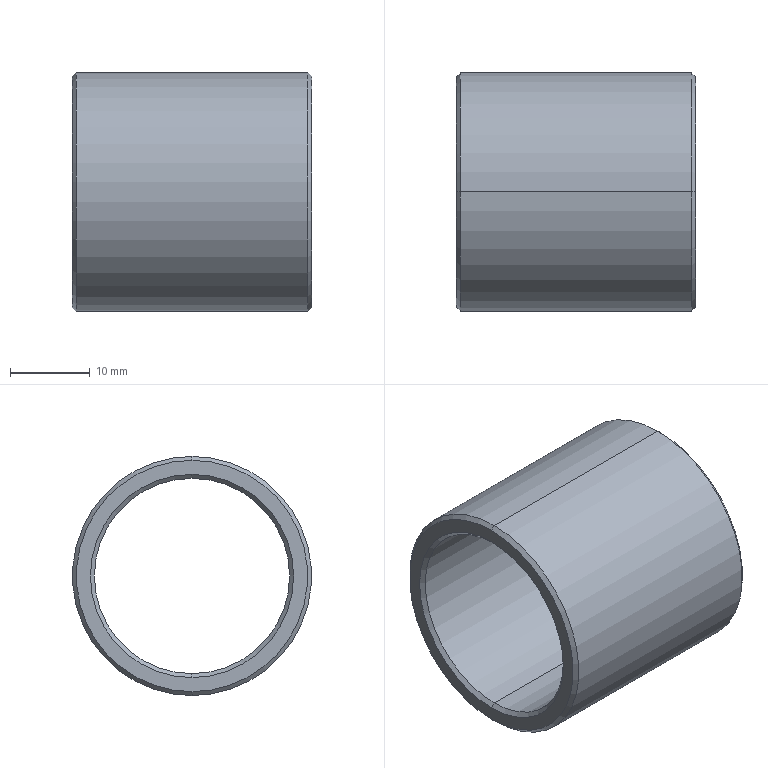Part | SolidWorks | features Revolution 1 | 1 solid | 14 faces | box 30 x 30 x 30 mm | volume 7020 mm3 | cone 8 | cylinder 4 | plane 2 | commonest cylinder face diameters 24.5 x2 30 x2
STEP:
#1=CARTESIAN_POINT('',(-14.5,0.,-12.25));
#2=VERTEX_POINT('',#1);
#3=CARTESIAN_POINT('',(-14.5,0.,12.25));
#4=VERTEX_POINT('',#3);
#5=CARTESIAN_POINT('',(-14.5,0.,0.));
#6=DIRECTION('',(-1.,0.,0.));
#7=DIRECTION('',(0.,0.,1.));
#8=AXIS2_PLACEMENT_3D('',#5,#6,#7);
#9=CIRCLE('',#8,12.25);
#10=EDGE_CURVE('',#2,#4,#9,.T.);
#11=ORIENTED_EDGE('',*,*,#10,.F.);
#12=CARTESIAN_POINT('',(-15.,0.,-12.75));
#13=VERTEX_POINT('',#12);
#14=CARTESIAN_POINT('',(-15.,0.,-12.75));
#15=DIRECTION('',(-0.7071,0.,-0.7071));
#16=VECTOR('',#15,1000.);
#17=LINE('',#14,#16);
#18=EDGE_CURVE('',#2,#13,#17,.T.);
#19=ORIENTED_EDGE('',*,*,#18,.T.);
#20=CARTESIAN_POINT('',(-15.,0.,12.75));
#21=VERTEX_POINT('',#20);
#22=CARTESIAN_POINT('',(-15.,0.,0.));
#23=DIRECTION('',(-1.,0.,0.));
#24=DIRECTION('',(0.,0.,1.));
#25=AXIS2_PLACEMENT_3D('',#22,#23,#24);
#26=CIRCLE('',#25,12.75);
#27=EDGE_CURVE('',#13,#21,#26,.T.);
#28=ORIENTED_EDGE('',*,*,#27,.T.);
#29=CARTESIAN_POINT('',(-15.,0.,12.75));
#30=DIRECTION('',(-0.7071,0.,0.7071));
#31=VECTOR('',#30,1000.);
#32=LINE('',#29,#31);
#33=EDGE_CURVE('',#4,#21,#32,.T.);
#34=ORIENTED_EDGE('',*,*,#33,.F.);
#35=EDGE_LOOP('',(#11,#19,#28,#34));
#36=FACE_OUTER_BOUND('',#35,.T.);
#37=CARTESIAN_POINT('',(-15.,0.,0.));
#38=DIRECTION('',(-1.,0.,0.));
#39=DIRECTION('',(0.,0.,1.));
#40=AXIS2_PLACEMENT_3D('',#37,#38,#39);
#41=CONICAL_SURFACE('',#40,12.75,0.7854);
#42=ADVANCED_FACE('',(#36),#41,.F.);
#43=CARTESIAN_POINT('',(14.5,0.,-12.25));
#44=VERTEX_POINT('',#43);
#45=CARTESIAN_POINT('',(14.5,0.,12.25));
#46=VERTEX_POINT('',#45);
#47=CARTESIAN_POINT('',(14.5,0.,0.));
#48=DIRECTION('',(-1.,0.,0.));
#49=DIRECTION('',(0.,0.,1.));
#50=AXIS2_PLACEMENT_3D('',#47,#48,#49);
#51=CIRCLE('',#50,12.25);
#52=EDGE_CURVE('',#44,#46,#51,.T.);
#53=ORIENTED_EDGE('',*,*,#52,.F.);
#54=CARTESIAN_POINT('',(-1000.,0.,-12.25));
#55=DIRECTION('',(-1.,0.,0.));
#56=VECTOR('',#55,1000.);
#57=LINE('',#54,#56);
#58=EDGE_CURVE('',#44,#2,#57,.T.);
#59=ORIENTED_EDGE('',*,*,#58,.T.);
#60=ORIENTED_EDGE('',*,*,#10,.T.);
#61=CARTESIAN_POINT('',(-1000.,0.,12.25));
#62=DIRECTION('',(-1.,0.,0.));
#63=VECTOR('',#62,1000.);
#64=LINE('',#61,#63);
#65=EDGE_CURVE('',#46,#4,#64,.T.);
#66=ORIENTED_EDGE('',*,*,#65,.F.);
#67=EDGE_LOOP('',(#53,#59,#60,#66));
#68=FACE_OUTER_BOUND('',#67,.T.);
#69=CARTESIAN_POINT('',(-1000.,0.,0.));
#70=DIRECTION('',(-1.,0.,0.));
#71=DIRECTION('',(0.,0.,1.));
#72=AXIS2_PLACEMENT_3D('',#69,#70,#71);
#73=CYLINDRICAL_SURFACE('',#72,12.25);
#74=ADVANCED_FACE('',(#68),#73,.F.);
#75=ORIENTED_EDGE('',*,*,#52,.T.);
#76=CARTESIAN_POINT('',(15.,0.,12.75));
#77=VERTEX_POINT('',#76);
#78=CARTESIAN_POINT('',(14.5,0.,12.25));
#79=DIRECTION('',(0.7071,0.,0.7071));
#80=VECTOR('',#79,1000.);
#81=LINE('',#78,#80);
#82=EDGE_CURVE('',#46,#77,#81,.T.);
#83=ORIENTED_EDGE('',*,*,#82,.T.);
#84=CARTESIAN_POINT('',(15.,0.,-12.75));
#85=VERTEX_POINT('',#84);
#86=CARTESIAN_POINT('',(15.,0.,0.));
#87=DIRECTION('',(-1.,0.,0.));
#88=DIRECTION('',(0.,0.,1.));
#89=AXIS2_PLACEMENT_3D('',#86,#87,#88);
#90=CIRCLE('',#89,12.75);
#91=EDGE_CURVE('',#85,#77,#90,.T.);
#92=ORIENTED_EDGE('',*,*,#91,.F.);
#93=CARTESIAN_POINT('',(14.5,0.,-12.25));
#94=DIRECTION('',(0.7071,0.,-0.7071));
#95=VECTOR('',#94,1000.);
#96=LINE('',#93,#95);
#97=EDGE_CURVE('',#44,#85,#96,.T.);
#98=ORIENTED_EDGE('',*,*,#97,.F.);
#99=EDGE_LOOP('',(#75,#83,#92,#98));
#100=FACE_OUTER_BOUND('',#99,.T.);
#101=CARTESIAN_POINT('',(14.5,0.,0.));
#102=DIRECTION('',(1.,0.,0.));
#103=DIRECTION('',(0.,0.,-1.));
#104=AXIS2_PLACEMENT_3D('',#101,#102,#103);
#105=CONICAL_SURFACE('',#104,12.25,0.7854);
#106=ADVANCED_FACE('',(#100),#105,.F.);
#107=CARTESIAN_POINT('',(15.,0.,14.5));
#108=VERTEX_POINT('',#107);
#109=CARTESIAN_POINT('',(15.,0.,-14.5));
#110=VERTEX_POINT('',#109);
#111=CARTESIAN_POINT('',(15.,0.,0.));
#112=DIRECTION('',(-1.,0.,0.));
#113=DIRECTION('',(0.,0.,1.));
#114=AXIS2_PLACEMENT_3D('',#111,#112,#113);
#115=CIRCLE('',#114,14.5);
#116=EDGE_CURVE('',#108,#110,#115,.T.);
#117=ORIENTED_EDGE('',*,*,#116,.T.);
#118=CARTESIAN_POINT('',(14.5,0.,-15.));
#119=VERTEX_POINT('',#118);
#120=CARTESIAN_POINT('',(15.,0.,-14.5));
#121=DIRECTION('',(-0.7071,0.,-0.7071));
#122=VECTOR('',#121,1000.);
#123=LINE('',#120,#122);
#124=EDGE_CURVE('',#110,#119,#123,.T.);
#125=ORIENTED_EDGE('',*,*,#124,.T.);
#126=CARTESIAN_POINT('',(14.5,0.,15.));
#127=VERTEX_POINT('',#126);
#128=CARTESIAN_POINT('',(14.5,0.,0.));
#129=DIRECTION('',(-1.,0.,0.));
#130=DIRECTION('',(0.,0.,1.));
#131=AXIS2_PLACEMENT_3D('',#128,#129,#130);
#132=CIRCLE('',#131,15.);
#133=EDGE_CURVE('',#127,#119,#132,.T.);
#134=ORIENTED_EDGE('',*,*,#133,.F.);
#135=CARTESIAN_POINT('',(15.,0.,14.5));
#136=DIRECTION('',(-0.7071,0.,0.7071));
#137=VECTOR('',#136,1000.);
#138=LINE('',#135,#137);
#139=EDGE_CURVE('',#108,#127,#138,.T.);
#140=ORIENTED_EDGE('',*,*,#139,.F.);
#141=EDGE_LOOP('',(#117,#125,#134,#140));
#142=FACE_OUTER_BOUND('',#141,.T.);
#143=CARTESIAN_POINT('',(15.,0.,0.));
#144=DIRECTION('',(-1.,0.,0.));
#145=DIRECTION('',(0.,0.,1.));
#146=AXIS2_PLACEMENT_3D('',#143,#144,#145);
#147=CONICAL_SURFACE('',#146,14.5,0.7854);
#148=ADVANCED_FACE('',(#142),#147,.T.);
#149=ORIENTED_EDGE('',*,*,#133,.T.);
#150=CARTESIAN_POINT('',(-14.5,0.,-15.));
#151=VERTEX_POINT('',#150);
#152=CARTESIAN_POINT('',(-1000.,0.,-15.));
#153=DIRECTION('',(-1.,0.,0.));
#154=VECTOR('',#153,1000.);
#155=LINE('',#152,#154);
#156=EDGE_CURVE('',#119,#151,#155,.T.);
#157=ORIENTED_EDGE('',*,*,#156,.T.);
#158=CARTESIAN_POINT('',(-14.5,0.,15.));
#159=VERTEX_POINT('',#158);
#160=CARTESIAN_POINT('',(-14.5,0.,0.));
#161=DIRECTION('',(-1.,0.,0.));
#162=DIRECTION('',(0.,0.,1.));
#163=AXIS2_PLACEMENT_3D('',#160,#161,#162);
#164=CIRCLE('',#163,15.);
#165=EDGE_CURVE('',#159,#151,#164,.T.);
#166=ORIENTED_EDGE('',*,*,#165,.F.);
#167=CARTESIAN_POINT('',(-1000.,0.,15.));
#168=DIRECTION('',(-1.,0.,0.));
#169=VECTOR('',#168,1000.);
#170=LINE('',#167,#169);
#171=EDGE_CURVE('',#127,#159,#170,.T.);
#172=ORIENTED_EDGE('',*,*,#171,.F.);
#173=EDGE_LOOP('',(#149,#157,#166,#172));
#174=FACE_OUTER_BOUND('',#173,.T.);
#175=CARTESIAN_POINT('',(-1000.,0.,0.));
#176=DIRECTION('',(-1.,0.,0.));
#177=DIRECTION('',(0.,0.,1.));
#178=AXIS2_PLACEMENT_3D('',#175,#176,#177);
#179=CYLINDRICAL_SURFACE('',#178,15.);
#180=ADVANCED_FACE('',(#174),#179,.T.);
#181=CARTESIAN_POINT('',(-15.,0.,14.5));
#182=VERTEX_POINT('',#181);
#183=CARTESIAN_POINT('',(-15.,0.,-14.5));
#184=VERTEX_POINT('',#183);
#185=CARTESIAN_POINT('',(-15.,0.,0.));
#186=DIRECTION('',(-1.,0.,0.));
#187=DIRECTION('',(0.,0.,1.));
#188=AXIS2_PLACEMENT_3D('',#185,#186,#187);
#189=CIRCLE('',#188,14.5);
#190=EDGE_CURVE('',#182,#184,#189,.T.);
#191=ORIENTED_EDGE('',*,*,#190,.F.);
#192=CARTESIAN_POINT('',(-14.5,0.,15.));
#193=DIRECTION('',(0.7071,0.,0.7071));
#194=VECTOR('',#193,1000.);
#195=LINE('',#192,#194);
#196=EDGE_CURVE('',#182,#159,#195,.T.);
#197=ORIENTED_EDGE('',*,*,#196,.T.);
#198=ORIENTED_EDGE('',*,*,#165,.T.);
#199=CARTESIAN_POINT('',(-14.5,0.,-15.));
#200=DIRECTION('',(0.7071,0.,-0.7071));
#201=VECTOR('',#200,1000.);
#202=LINE('',#199,#201);
#203=EDGE_CURVE('',#184,#151,#202,.T.);
#204=ORIENTED_EDGE('',*,*,#203,.F.);
#205=EDGE_LOOP('',(#191,#197,#198,#204));
#206=FACE_OUTER_BOUND('',#205,.T.);
#207=CARTESIAN_POINT('',(-14.5,0.,0.));
#208=DIRECTION('',(1.,0.,0.));
#209=DIRECTION('',(0.,0.,-1.));
#210=AXIS2_PLACEMENT_3D('',#207,#208,#209);
#211=CONICAL_SURFACE('',#210,15.,0.7854);
#212=ADVANCED_FACE('',(#206),#211,.T.);
#213=CARTESIAN_POINT('',(-15.,0.,0.));
#214=DIRECTION('',(-1.,0.,0.));
#215=DIRECTION('',(0.,0.,1.));
#216=AXIS2_PLACEMENT_3D('',#213,#214,#215);
#217=CIRCLE('',#216,12.75);
#218=EDGE_CURVE('',#21,#13,#217,.T.);
#219=ORIENTED_EDGE('',*,*,#218,.F.);
#220=ORIENTED_EDGE('',*,*,#27,.F.);
#221=EDGE_LOOP('',(#219,#220));
#222=FACE_BOUND('',#221,.T.);
#223=CARTESIAN_POINT('',(-15.,0.,0.));
#224=DIRECTION('',(-1.,0.,0.));
#225=DIRECTION('',(0.,0.,1.));
#226=AXIS2_PLACEMENT_3D('',#223,#224,#225);
#227=CIRCLE('',#226,14.5);
#228=EDGE_CURVE('',#184,#182,#227,.T.);
#229=ORIENTED_EDGE('',*,*,#228,.T.);
#230=ORIENTED_EDGE('',*,*,#190,.T.);
#231=EDGE_LOOP('',(#229,#230));
#232=FACE_OUTER_BOUND('',#231,.T.);
#233=CARTESIAN_POINT('',(-15.,0.,-12.75));
#234=DIRECTION('',(1.,0.,0.));
#235=DIRECTION('',(0.,0.,-1.));
#236=AXIS2_PLACEMENT_3D('',#233,#234,#235);
#237=PLANE('',#236);
#238=ADVANCED_FACE('',(#222,#232),#237,.F.);
#239=ORIENTED_EDGE('',*,*,#196,.F.);
#240=ORIENTED_EDGE('',*,*,#228,.F.);
#241=ORIENTED_EDGE('',*,*,#203,.T.);
#242=CARTESIAN_POINT('',(-14.5,0.,0.));
#243=DIRECTION('',(-1.,0.,0.));
#244=DIRECTION('',(0.,0.,1.));
#245=AXIS2_PLACEMENT_3D('',#242,#243,#244);
#246=CIRCLE('',#245,15.);
#247=EDGE_CURVE('',#151,#159,#246,.T.);
#248=ORIENTED_EDGE('',*,*,#247,.T.);
#249=EDGE_LOOP('',(#239,#240,#241,#248));
#250=FACE_OUTER_BOUND('',#249,.T.);
#251=CARTESIAN_POINT('',(-14.5,0.,0.));
#252=DIRECTION('',(1.,0.,0.));
#253=DIRECTION('',(0.,0.,-1.));
#254=AXIS2_PLACEMENT_3D('',#251,#252,#253);
#255=CONICAL_SURFACE('',#254,15.,0.7854);
#256=ADVANCED_FACE('',(#250),#255,.T.);
#257=ORIENTED_EDGE('',*,*,#156,.F.);
#258=CARTESIAN_POINT('',(14.5,0.,0.));
#259=DIRECTION('',(-1.,0.,0.));
#260=DIRECTION('',(0.,0.,1.));
#261=AXIS2_PLACEMENT_3D('',#258,#259,#260);
#262=CIRCLE('',#261,15.);
#263=EDGE_CURVE('',#119,#127,#262,.T.);
#264=ORIENTED_EDGE('',*,*,#263,.T.);
#265=ORIENTED_EDGE('',*,*,#171,.T.);
#266=ORIENTED_EDGE('',*,*,#247,.F.);
#267=EDGE_LOOP('',(#257,#264,#265,#266));
#268=FACE_OUTER_BOUND('',#267,.T.);
#269=CARTESIAN_POINT('',(-1000.,0.,0.));
#270=DIRECTION('',(-1.,0.,0.));
#271=DIRECTION('',(0.,0.,1.));
#272=AXIS2_PLACEMENT_3D('',#269,#270,#271);
#273=CYLINDRICAL_SURFACE('',#272,15.);
#274=ADVANCED_FACE('',(#268),#273,.T.);
#275=ORIENTED_EDGE('',*,*,#124,.F.);
#276=CARTESIAN_POINT('',(15.,0.,0.));
#277=DIRECTION('',(-1.,0.,0.));
#278=DIRECTION('',(0.,0.,1.));
#279=AXIS2_PLACEMENT_3D('',#276,#277,#278);
#280=CIRCLE('',#279,14.5);
#281=EDGE_CURVE('',#110,#108,#280,.T.);
#282=ORIENTED_EDGE('',*,*,#281,.T.);
#283=ORIENTED_EDGE('',*,*,#139,.T.);
#284=ORIENTED_EDGE('',*,*,#263,.F.);
#285=EDGE_LOOP('',(#275,#282,#283,#284));
#286=FACE_OUTER_BOUND('',#285,.T.);
#287=CARTESIAN_POINT('',(15.,0.,0.));
#288=DIRECTION('',(-1.,0.,0.));
#289=DIRECTION('',(0.,0.,1.));
#290=AXIS2_PLACEMENT_3D('',#287,#288,#289);
#291=CONICAL_SURFACE('',#290,14.5,0.7854);
#292=ADVANCED_FACE('',(#286),#291,.T.);
#293=ORIENTED_EDGE('',*,*,#116,.F.);
#294=ORIENTED_EDGE('',*,*,#281,.F.);
#295=EDGE_LOOP('',(#293,#294));
#296=FACE_OUTER_BOUND('',#295,.T.);
#297=ORIENTED_EDGE('',*,*,#91,.T.);
#298=CARTESIAN_POINT('',(15.,0.,0.));
#299=DIRECTION('',(-1.,0.,0.));
#300=DIRECTION('',(0.,0.,1.));
#301=AXIS2_PLACEMENT_3D('',#298,#299,#300);
#302=CIRCLE('',#301,12.75);
#303=EDGE_CURVE('',#77,#85,#302,.T.);
#304=ORIENTED_EDGE('',*,*,#303,.T.);
#305=EDGE_LOOP('',(#297,#304));
#306=FACE_BOUND('',#305,.T.);
#307=CARTESIAN_POINT('',(15.,0.,-12.75));
#308=DIRECTION('',(-1.,0.,0.));
#309=DIRECTION('',(0.,0.,1.));
#310=AXIS2_PLACEMENT_3D('',#307,#308,#309);
#311=PLANE('',#310);
#312=ADVANCED_FACE('',(#296,#306),#311,.F.);
#313=ORIENTED_EDGE('',*,*,#82,.F.);
#314=CARTESIAN_POINT('',(14.5,0.,0.));
#315=DIRECTION('',(-1.,0.,0.));
#316=DIRECTION('',(0.,0.,1.));
#317=AXIS2_PLACEMENT_3D('',#314,#315,#316);
#318=CIRCLE('',#317,12.25);
#319=EDGE_CURVE('',#46,#44,#318,.T.);
#320=ORIENTED_EDGE('',*,*,#319,.T.);
#321=ORIENTED_EDGE('',*,*,#97,.T.);
#322=ORIENTED_EDGE('',*,*,#303,.F.);
#323=EDGE_LOOP('',(#313,#320,#321,#322));
#324=FACE_OUTER_BOUND('',#323,.T.);
#325=CARTESIAN_POINT('',(14.5,0.,0.));
#326=DIRECTION('',(1.,0.,0.));
#327=DIRECTION('',(0.,0.,-1.));
#328=AXIS2_PLACEMENT_3D('',#325,#326,#327);
#329=CONICAL_SURFACE('',#328,12.25,0.7854);
#330=ADVANCED_FACE('',(#324),#329,.F.);
#331=ORIENTED_EDGE('',*,*,#58,.F.);
#332=ORIENTED_EDGE('',*,*,#319,.F.);
#333=ORIENTED_EDGE('',*,*,#65,.T.);
#334=CARTESIAN_POINT('',(-14.5,0.,0.));
#335=DIRECTION('',(-1.,0.,0.));
#336=DIRECTION('',(0.,0.,1.));
#337=AXIS2_PLACEMENT_3D('',#334,#335,#336);
#338=CIRCLE('',#337,12.25);
#339=EDGE_CURVE('',#4,#2,#338,.T.);
#340=ORIENTED_EDGE('',*,*,#339,.T.);
#341=EDGE_LOOP('',(#331,#332,#333,#340));
#342=FACE_OUTER_BOUND('',#341,.T.);
#343=CARTESIAN_POINT('',(-1000.,0.,0.));
#344=DIRECTION('',(-1.,0.,0.));
#345=DIRECTION('',(0.,0.,1.));
#346=AXIS2_PLACEMENT_3D('',#343,#344,#345);
#347=CYLINDRICAL_SURFACE('',#346,12.25);
#348=ADVANCED_FACE('',(#342),#347,.F.);
#349=ORIENTED_EDGE('',*,*,#18,.F.);
#350=ORIENTED_EDGE('',*,*,#339,.F.);
#351=ORIENTED_EDGE('',*,*,#33,.T.);
#352=ORIENTED_EDGE('',*,*,#218,.T.);
#353=EDGE_LOOP('',(#349,#350,#351,#352));
#354=FACE_OUTER_BOUND('',#353,.T.);
#355=CARTESIAN_POINT('',(-15.,0.,0.));
#356=DIRECTION('',(-1.,0.,0.));
#357=DIRECTION('',(0.,0.,1.));
#358=AXIS2_PLACEMENT_3D('',#355,#356,#357);
#359=CONICAL_SURFACE('',#358,12.75,0.7854);
#360=ADVANCED_FACE('',(#354),#359,.F.);
#361=CLOSED_SHELL('',(#42,#74,#106,#148,#180,#212,#238,#256,#274,#292,#312,#330,#348,#360));
#362=MANIFOLD_SOLID_BREP('',#361);
#363=CARTESIAN_POINT('',(0.,0.,0.));
#364=DIRECTION('',(0.,0.,1.));
#365=DIRECTION('',(1.,0.,0.));
#366=AXIS2_PLACEMENT_3D('',#363,#364,#365);
#367=(LENGTH_UNIT()NAMED_UNIT(*)SI_UNIT(.MILLI.,.METRE.));
#368=UNCERTAINTY_MEASURE_WITH_UNIT(LENGTH_MEASURE(0.00001),#367,'','');
#369=(NAMED_UNIT(*)PLANE_ANGLE_UNIT()SI_UNIT($,.RADIAN.));
#370=(NAMED_UNIT(*)SI_UNIT($,.STERADIAN.)SOLID_ANGLE_UNIT());
#371=(GEOMETRIC_REPRESENTATION_CONTEXT(3)GLOBAL_UNCERTAINTY_ASSIGNED_CONTEXT((#368))GLOBAL_UNIT_ASSIGNED_CONTEXT((#367,#369,#370))REPRESENTATION_CONTEXT('',''));
#372=ADVANCED_BREP_SHAPE_REPRESENTATION('',(#362,#366),#371);